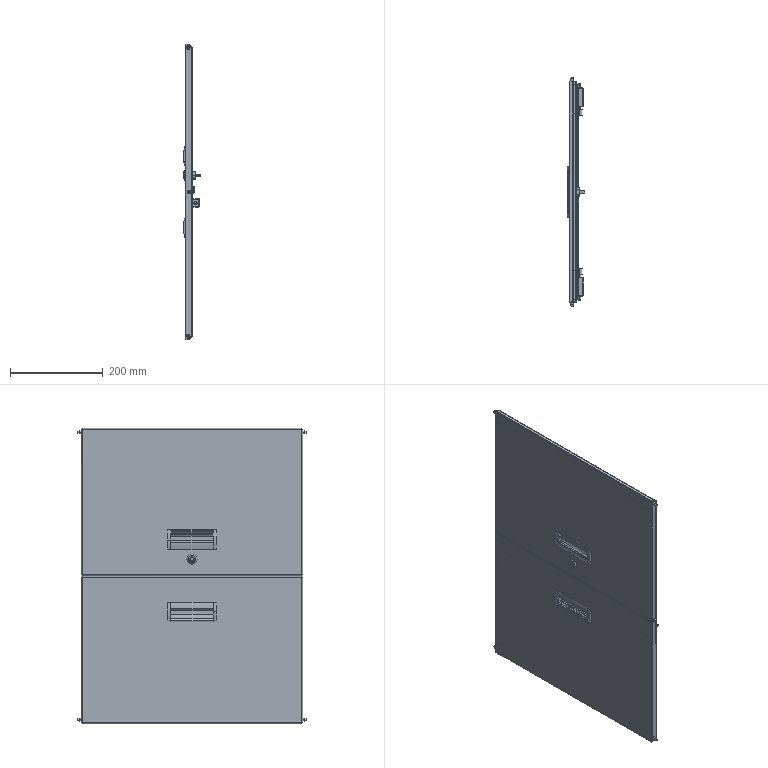Part | SolidWorks | 25 solids | 704 faces | box 37.5 x 494 x 636 mm | volume 633113 mm3 | plane 394 | cylinder 280 | cone 14 | torus 8 | spline 8 | commonest cylinder face diameters 1 x36 7 x23 0.6 x21 2.5 x16 3.2 x16 5.5 x16